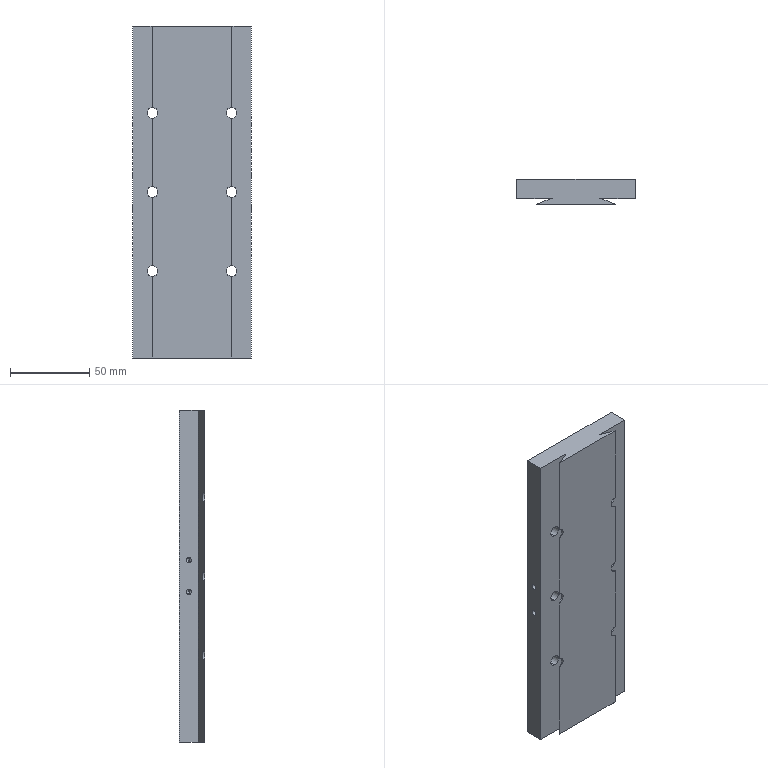Part | SolidWorks | features HoleWzd 2, Extrusion 1, LPattern 1, MirrorPattern 1 | 1 solid | 44 faces | box 75 x 16 x 210 mm | volume 219565 mm3 | cylinder 26 | plane 10 | cone 8 | commonest cylinder face diameters 6.8 x18 3.3 x8
STEP:
#1=CARTESIAN_POINT('',(25.,-6.,46.6));
#2=VERTEX_POINT('',#1);
#3=CARTESIAN_POINT('',(25.,-6.,53.4));
#4=VERTEX_POINT('',#3);
#5=CARTESIAN_POINT('',(25.,-6.,50.));
#6=DIRECTION('',(0.,1.,0.));
#7=DIRECTION('',(0.,0.,1.));
#8=AXIS2_PLACEMENT_3D('',#5,#6,#7);
#9=CIRCLE('',#8,3.4);
#10=EDGE_CURVE('',#2,#4,#9,.T.);
#11=ORIENTED_EDGE('',*,*,#10,.F.);
#12=CARTESIAN_POINT('',(25.,6.,46.6));
#13=VERTEX_POINT('',#12);
#14=CARTESIAN_POINT('',(25.,6.,46.6));
#15=DIRECTION('',(0.,1.,0.));
#16=VECTOR('',#15,1000.);
#17=LINE('',#14,#16);
#18=EDGE_CURVE('',#2,#13,#17,.T.);
#19=ORIENTED_EDGE('',*,*,#18,.T.);
#20=CARTESIAN_POINT('',(25.,6.,53.4));
#21=VERTEX_POINT('',#20);
#22=CARTESIAN_POINT('',(25.,6.,50.));
#23=DIRECTION('',(0.,1.,0.));
#24=DIRECTION('',(0.,0.,1.));
#25=AXIS2_PLACEMENT_3D('',#22,#23,#24);
#26=CIRCLE('',#25,3.4);
#27=EDGE_CURVE('',#13,#21,#26,.T.);
#28=ORIENTED_EDGE('',*,*,#27,.T.);
#29=CARTESIAN_POINT('',(25.,6.,53.4));
#30=DIRECTION('',(0.,1.,0.));
#31=VECTOR('',#30,1000.);
#32=LINE('',#29,#31);
#33=EDGE_CURVE('',#4,#21,#32,.T.);
#34=ORIENTED_EDGE('',*,*,#33,.F.);
#35=EDGE_LOOP('',(#11,#19,#28,#34));
#36=FACE_OUTER_BOUND('',#35,.T.);
#37=CARTESIAN_POINT('',(25.,6.,50.));
#38=DIRECTION('',(0.,1.,0.));
#39=DIRECTION('',(0.,0.,1.));
#40=AXIS2_PLACEMENT_3D('',#37,#38,#39);
#41=CYLINDRICAL_SURFACE('',#40,3.4);
#42=ADVANCED_FACE('',(#36),#41,.F.);
#43=CARTESIAN_POINT('',(-25.,-6.,46.6));
#44=VERTEX_POINT('',#43);
#45=CARTESIAN_POINT('',(-25.,-6.,53.4));
#46=VERTEX_POINT('',#45);
#47=CARTESIAN_POINT('',(-25.,-6.,50.));
#48=DIRECTION('',(0.,1.,0.));
#49=DIRECTION('',(0.,0.,1.));
#50=AXIS2_PLACEMENT_3D('',#47,#48,#49);
#51=CIRCLE('',#50,3.4);
#52=EDGE_CURVE('',#44,#46,#51,.T.);
#53=ORIENTED_EDGE('',*,*,#52,.F.);
#54=CARTESIAN_POINT('',(-25.,6.,46.6));
#55=VERTEX_POINT('',#54);
#56=CARTESIAN_POINT('',(-25.,6.,46.6));
#57=DIRECTION('',(0.,1.,0.));
#58=VECTOR('',#57,1000.);
#59=LINE('',#56,#58);
#60=EDGE_CURVE('',#44,#55,#59,.T.);
#61=ORIENTED_EDGE('',*,*,#60,.T.);
#62=CARTESIAN_POINT('',(-25.,6.,53.4));
#63=VERTEX_POINT('',#62);
#64=CARTESIAN_POINT('',(-25.,6.,50.));
#65=DIRECTION('',(0.,1.,0.));
#66=DIRECTION('',(0.,0.,1.));
#67=AXIS2_PLACEMENT_3D('',#64,#65,#66);
#68=CIRCLE('',#67,3.4);
#69=EDGE_CURVE('',#55,#63,#68,.T.);
#70=ORIENTED_EDGE('',*,*,#69,.T.);
#71=CARTESIAN_POINT('',(-25.,6.,53.4));
#72=DIRECTION('',(0.,1.,0.));
#73=VECTOR('',#72,1000.);
#74=LINE('',#71,#73);
#75=EDGE_CURVE('',#46,#63,#74,.T.);
#76=ORIENTED_EDGE('',*,*,#75,.F.);
#77=EDGE_LOOP('',(#53,#61,#70,#76));
#78=FACE_OUTER_BOUND('',#77,.T.);
#79=CARTESIAN_POINT('',(-25.,6.,50.));
#80=DIRECTION('',(0.,1.,0.));
#81=DIRECTION('',(0.,0.,1.));
#82=AXIS2_PLACEMENT_3D('',#79,#80,#81);
#83=CYLINDRICAL_SURFACE('',#82,3.4);
#84=ADVANCED_FACE('',(#78),#83,.F.);
#85=CARTESIAN_POINT('',(25.,-6.,-3.4));
#86=VERTEX_POINT('',#85);
#87=CARTESIAN_POINT('',(25.,-6.,3.4));
#88=VERTEX_POINT('',#87);
#89=CARTESIAN_POINT('',(25.,-6.,0.));
#90=DIRECTION('',(0.,1.,0.));
#91=DIRECTION('',(0.,0.,1.));
#92=AXIS2_PLACEMENT_3D('',#89,#90,#91);
#93=CIRCLE('',#92,3.4);
#94=EDGE_CURVE('',#86,#88,#93,.T.);
#95=ORIENTED_EDGE('',*,*,#94,.F.);
#96=CARTESIAN_POINT('',(25.,6.,-3.4));
#97=VERTEX_POINT('',#96);
#98=CARTESIAN_POINT('',(25.,6.,-3.4));
#99=DIRECTION('',(0.,1.,0.));
#100=VECTOR('',#99,1000.);
#101=LINE('',#98,#100);
#102=EDGE_CURVE('',#86,#97,#101,.T.);
#103=ORIENTED_EDGE('',*,*,#102,.T.);
#104=CARTESIAN_POINT('',(25.,6.,3.4));
#105=VERTEX_POINT('',#104);
#106=CARTESIAN_POINT('',(25.,6.,0.));
#107=DIRECTION('',(0.,1.,0.));
#108=DIRECTION('',(0.,0.,1.));
#109=AXIS2_PLACEMENT_3D('',#106,#107,#108);
#110=CIRCLE('',#109,3.4);
#111=EDGE_CURVE('',#97,#105,#110,.T.);
#112=ORIENTED_EDGE('',*,*,#111,.T.);
#113=CARTESIAN_POINT('',(25.,6.,3.4));
#114=DIRECTION('',(0.,1.,0.));
#115=VECTOR('',#114,1000.);
#116=LINE('',#113,#115);
#117=EDGE_CURVE('',#88,#105,#116,.T.);
#118=ORIENTED_EDGE('',*,*,#117,.F.);
#119=EDGE_LOOP('',(#95,#103,#112,#118));
#120=FACE_OUTER_BOUND('',#119,.T.);
#121=CARTESIAN_POINT('',(25.,6.,0.));
#122=DIRECTION('',(0.,1.,0.));
#123=DIRECTION('',(0.,0.,1.));
#124=AXIS2_PLACEMENT_3D('',#121,#122,#123);
#125=CYLINDRICAL_SURFACE('',#124,3.4);
#126=ADVANCED_FACE('',(#120),#125,.F.);
#127=CARTESIAN_POINT('',(-25.,-6.,-3.4));
#128=VERTEX_POINT('',#127);
#129=CARTESIAN_POINT('',(-25.,-6.,3.4));
#130=VERTEX_POINT('',#129);
#131=CARTESIAN_POINT('',(-25.,-6.,0.));
#132=DIRECTION('',(0.,1.,0.));
#133=DIRECTION('',(0.,0.,1.));
#134=AXIS2_PLACEMENT_3D('',#131,#132,#133);
#135=CIRCLE('',#134,3.4);
#136=EDGE_CURVE('',#128,#130,#135,.T.);
#137=ORIENTED_EDGE('',*,*,#136,.F.);
#138=CARTESIAN_POINT('',(-25.,6.,-3.4));
#139=VERTEX_POINT('',#138);
#140=CARTESIAN_POINT('',(-25.,6.,-3.4));
#141=DIRECTION('',(0.,1.,0.));
#142=VECTOR('',#141,1000.);
#143=LINE('',#140,#142);
#144=EDGE_CURVE('',#128,#139,#143,.T.);
#145=ORIENTED_EDGE('',*,*,#144,.T.);
#146=CARTESIAN_POINT('',(-25.,6.,3.4));
#147=VERTEX_POINT('',#146);
#148=CARTESIAN_POINT('',(-25.,6.,0.));
#149=DIRECTION('',(0.,1.,0.));
#150=DIRECTION('',(0.,0.,1.));
#151=AXIS2_PLACEMENT_3D('',#148,#149,#150);
#152=CIRCLE('',#151,3.4);
#153=EDGE_CURVE('',#139,#147,#152,.T.);
#154=ORIENTED_EDGE('',*,*,#153,.T.);
#155=CARTESIAN_POINT('',(-25.,6.,3.4));
#156=DIRECTION('',(0.,1.,0.));
#157=VECTOR('',#156,1000.);
#158=LINE('',#155,#157);
#159=EDGE_CURVE('',#130,#147,#158,.T.);
#160=ORIENTED_EDGE('',*,*,#159,.F.);
#161=EDGE_LOOP('',(#137,#145,#154,#160));
#162=FACE_OUTER_BOUND('',#161,.T.);
#163=CARTESIAN_POINT('',(-25.,6.,0.));
#164=DIRECTION('',(0.,1.,0.));
#165=DIRECTION('',(0.,0.,1.));
#166=AXIS2_PLACEMENT_3D('',#163,#164,#165);
#167=CYLINDRICAL_SURFACE('',#166,3.4);
#168=ADVANCED_FACE('',(#162),#167,.F.);
#169=CARTESIAN_POINT('',(25.,-6.,-53.4));
#170=VERTEX_POINT('',#169);
#171=CARTESIAN_POINT('',(25.,-6.,-46.6));
#172=VERTEX_POINT('',#171);
#173=CARTESIAN_POINT('',(25.,-6.,-50.));
#174=DIRECTION('',(0.,1.,0.));
#175=DIRECTION('',(0.,0.,1.));
#176=AXIS2_PLACEMENT_3D('',#173,#174,#175);
#177=CIRCLE('',#176,3.4);
#178=EDGE_CURVE('',#170,#172,#177,.T.);
#179=ORIENTED_EDGE('',*,*,#178,.F.);
#180=CARTESIAN_POINT('',(25.,6.,-53.4));
#181=VERTEX_POINT('',#180);
#182=CARTESIAN_POINT('',(25.,6.,-53.4));
#183=DIRECTION('',(0.,1.,0.));
#184=VECTOR('',#183,1000.);
#185=LINE('',#182,#184);
#186=EDGE_CURVE('',#170,#181,#185,.T.);
#187=ORIENTED_EDGE('',*,*,#186,.T.);
#188=CARTESIAN_POINT('',(25.,6.,-46.6));
#189=VERTEX_POINT('',#188);
#190=CARTESIAN_POINT('',(25.,6.,-50.));
#191=DIRECTION('',(0.,1.,0.));
#192=DIRECTION('',(0.,0.,1.));
#193=AXIS2_PLACEMENT_3D('',#190,#191,#192);
#194=CIRCLE('',#193,3.4);
#195=EDGE_CURVE('',#181,#189,#194,.T.);
#196=ORIENTED_EDGE('',*,*,#195,.T.);
#197=CARTESIAN_POINT('',(25.,6.,-46.6));
#198=DIRECTION('',(0.,1.,0.));
#199=VECTOR('',#198,1000.);
#200=LINE('',#197,#199);
#201=EDGE_CURVE('',#172,#189,#200,.T.);
#202=ORIENTED_EDGE('',*,*,#201,.F.);
#203=EDGE_LOOP('',(#179,#187,#196,#202));
#204=FACE_OUTER_BOUND('',#203,.T.);
#205=CARTESIAN_POINT('',(25.,6.,-50.));
#206=DIRECTION('',(0.,1.,0.));
#207=DIRECTION('',(0.,0.,1.));
#208=AXIS2_PLACEMENT_3D('',#205,#206,#207);
#209=CYLINDRICAL_SURFACE('',#208,3.4);
#210=ADVANCED_FACE('',(#204),#209,.F.);
#211=CARTESIAN_POINT('',(-25.,-6.,-53.4));
#212=VERTEX_POINT('',#211);
#213=CARTESIAN_POINT('',(-25.,-6.,-46.6));
#214=VERTEX_POINT('',#213);
#215=CARTESIAN_POINT('',(-25.,-6.,-50.));
#216=DIRECTION('',(0.,1.,0.));
#217=DIRECTION('',(0.,0.,1.));
#218=AXIS2_PLACEMENT_3D('',#215,#216,#217);
#219=CIRCLE('',#218,3.4);
#220=EDGE_CURVE('',#212,#214,#219,.T.);
#221=ORIENTED_EDGE('',*,*,#220,.F.);
#222=CARTESIAN_POINT('',(-25.,6.,-53.4));
#223=VERTEX_POINT('',#222);
#224=CARTESIAN_POINT('',(-25.,6.,-53.4));
#225=DIRECTION('',(0.,1.,0.));
#226=VECTOR('',#225,1000.);
#227=LINE('',#224,#226);
#228=EDGE_CURVE('',#212,#223,#227,.T.);
#229=ORIENTED_EDGE('',*,*,#228,.T.);
#230=CARTESIAN_POINT('',(-25.,6.,-46.6));
#231=VERTEX_POINT('',#230);
#232=CARTESIAN_POINT('',(-25.,6.,-50.));
#233=DIRECTION('',(0.,1.,0.));
#234=DIRECTION('',(0.,0.,1.));
#235=AXIS2_PLACEMENT_3D('',#232,#233,#234);
#236=CIRCLE('',#235,3.4);
#237=EDGE_CURVE('',#223,#231,#236,.T.);
#238=ORIENTED_EDGE('',*,*,#237,.T.);
#239=CARTESIAN_POINT('',(-25.,6.,-46.6));
#240=DIRECTION('',(0.,1.,0.));
#241=VECTOR('',#240,1000.);
#242=LINE('',#239,#241);
#243=EDGE_CURVE('',#214,#231,#242,.T.);
#244=ORIENTED_EDGE('',*,*,#243,.F.);
#245=EDGE_LOOP('',(#221,#229,#238,#244));
#246=FACE_OUTER_BOUND('',#245,.T.);
#247=CARTESIAN_POINT('',(-25.,6.,-50.));
#248=DIRECTION('',(0.,1.,0.));
#249=DIRECTION('',(0.,0.,1.));
#250=AXIS2_PLACEMENT_3D('',#247,#248,#249);
#251=CYLINDRICAL_SURFACE('',#250,3.4);
#252=ADVANCED_FACE('',(#246),#251,.F.);
#253=CARTESIAN_POINT('',(27.4,0.,-8.35));
#254=VERTEX_POINT('',#253);
#255=CARTESIAN_POINT('',(27.4,0.,-11.65));
#256=VERTEX_POINT('',#255);
#257=CARTESIAN_POINT('',(27.4,0.,-10.));
#258=DIRECTION('',(1.,0.,0.));
#259=DIRECTION('',(0.,0.,-1.));
#260=AXIS2_PLACEMENT_3D('',#257,#258,#259);
#261=CIRCLE('',#260,1.65);
#262=EDGE_CURVE('',#254,#256,#261,.T.);
#263=ORIENTED_EDGE('',*,*,#262,.F.);
#264=CARTESIAN_POINT('',(37.5,0.,-8.35));
#265=VERTEX_POINT('',#264);
#266=CARTESIAN_POINT('',(37.5,0.,-8.35));
#267=DIRECTION('',(1.,0.,0.));
#268=VECTOR('',#267,1000.);
#269=LINE('',#266,#268);
#270=EDGE_CURVE('',#254,#265,#269,.T.);
#271=ORIENTED_EDGE('',*,*,#270,.T.);
#272=CARTESIAN_POINT('',(37.5,0.,-11.65));
#273=VERTEX_POINT('',#272);
#274=CARTESIAN_POINT('',(37.5,0.,-10.));
#275=DIRECTION('',(1.,0.,0.));
#276=DIRECTION('',(0.,0.,-1.));
#277=AXIS2_PLACEMENT_3D('',#274,#275,#276);
#278=CIRCLE('',#277,1.65);
#279=EDGE_CURVE('',#265,#273,#278,.T.);
#280=ORIENTED_EDGE('',*,*,#279,.T.);
#281=CARTESIAN_POINT('',(37.5,0.,-11.65));
#282=DIRECTION('',(1.,0.,0.));
#283=VECTOR('',#282,1000.);
#284=LINE('',#281,#283);
#285=EDGE_CURVE('',#256,#273,#284,.T.);
#286=ORIENTED_EDGE('',*,*,#285,.F.);
#287=EDGE_LOOP('',(#263,#271,#280,#286));
#288=FACE_OUTER_BOUND('',#287,.T.);
#289=CARTESIAN_POINT('',(37.5,0.,-10.));
#290=DIRECTION('',(1.,0.,0.));
#291=DIRECTION('',(0.,0.,-1.));
#292=AXIS2_PLACEMENT_3D('',#289,#290,#291);
#293=CYLINDRICAL_SURFACE('',#292,1.65);
#294=ADVANCED_FACE('',(#288),#293,.F.);
#295=CARTESIAN_POINT('',(26.409,0.,-10.));
#296=VERTEX_POINT('',#295);
#297=CARTESIAN_POINT('',(27.4,0.,-11.65));
#298=DIRECTION('',(0.515,0.,-0.8572));
#299=VECTOR('',#298,1000.);
#300=LINE('',#297,#299);
#301=EDGE_CURVE('',#296,#256,#300,.T.);
#302=ORIENTED_EDGE('',*,*,#301,.F.);
#303=CARTESIAN_POINT('',(27.4,0.,-8.35));
#304=DIRECTION('',(0.515,0.,0.8572));
#305=VECTOR('',#304,1000.);
#306=LINE('',#303,#305);
#307=EDGE_CURVE('',#296,#254,#306,.T.);
#308=ORIENTED_EDGE('',*,*,#307,.T.);
#309=ORIENTED_EDGE('',*,*,#262,.T.);
#310=EDGE_LOOP('',(#302,#308,#309));
#311=FACE_OUTER_BOUND('',#310,.T.);
#312=CARTESIAN_POINT('',(27.4,0.,-10.));
#313=DIRECTION('',(1.,0.,0.));
#314=DIRECTION('',(0.,0.,-1.));
#315=AXIS2_PLACEMENT_3D('',#312,#313,#314);
#316=CONICAL_SURFACE('',#315,1.65,1.03);
#317=ADVANCED_FACE('',(#311),#316,.F.);
#318=CARTESIAN_POINT('',(27.4,0.,11.65));
#319=VERTEX_POINT('',#318);
#320=CARTESIAN_POINT('',(27.4,0.,8.35));
#321=VERTEX_POINT('',#320);
#322=CARTESIAN_POINT('',(27.4,0.,10.));
#323=DIRECTION('',(1.,0.,0.));
#324=DIRECTION('',(0.,0.,-1.));
#325=AXIS2_PLACEMENT_3D('',#322,#323,#324);
#326=CIRCLE('',#325,1.65);
#327=EDGE_CURVE('',#319,#321,#326,.T.);
#328=ORIENTED_EDGE('',*,*,#327,.F.);
#329=CARTESIAN_POINT('',(37.5,0.,11.65));
#330=VERTEX_POINT('',#329);
#331=CARTESIAN_POINT('',(37.5,0.,11.65));
#332=DIRECTION('',(1.,0.,0.));
#333=VECTOR('',#332,1000.);
#334=LINE('',#331,#333);
#335=EDGE_CURVE('',#319,#330,#334,.T.);
#336=ORIENTED_EDGE('',*,*,#335,.T.);
#337=CARTESIAN_POINT('',(37.5,0.,8.35));
#338=VERTEX_POINT('',#337);
#339=CARTESIAN_POINT('',(37.5,0.,10.));
#340=DIRECTION('',(1.,0.,0.));
#341=DIRECTION('',(0.,0.,-1.));
#342=AXIS2_PLACEMENT_3D('',#339,#340,#341);
#343=CIRCLE('',#342,1.65);
#344=EDGE_CURVE('',#330,#338,#343,.T.);
#345=ORIENTED_EDGE('',*,*,#344,.T.);
#346=CARTESIAN_POINT('',(37.5,0.,8.35));
#347=DIRECTION('',(1.,0.,0.));
#348=VECTOR('',#347,1000.);
#349=LINE('',#346,#348);
#350=EDGE_CURVE('',#321,#338,#349,.T.);
#351=ORIENTED_EDGE('',*,*,#350,.F.);
#352=EDGE_LOOP('',(#328,#336,#345,#351));
#353=FACE_OUTER_BOUND('',#352,.T.);
#354=CARTESIAN_POINT('',(37.5,0.,10.));
#355=DIRECTION('',(1.,0.,0.));
#356=DIRECTION('',(0.,0.,-1.));
#357=AXIS2_PLACEMENT_3D('',#354,#355,#356);
#358=CYLINDRICAL_SURFACE('',#357,1.65);
#359=ADVANCED_FACE('',(#353),#358,.F.);
#360=CARTESIAN_POINT('',(26.409,0.,10.));
#361=VERTEX_POINT('',#360);
#362=CARTESIAN_POINT('',(27.4,0.,8.35));
#363=DIRECTION('',(0.515,0.,-0.8572));
#364=VECTOR('',#363,1000.);
#365=LINE('',#362,#364);
#366=EDGE_CURVE('',#361,#321,#365,.T.);
#367=ORIENTED_EDGE('',*,*,#366,.F.);
#368=CARTESIAN_POINT('',(27.4,0.,11.65));
#369=DIRECTION('',(0.515,0.,0.8572));
#370=VECTOR('',#369,1000.);
#371=LINE('',#368,#370);
#372=EDGE_CURVE('',#361,#319,#371,.T.);
#373=ORIENTED_EDGE('',*,*,#372,.T.);
#374=ORIENTED_EDGE('',*,*,#327,.T.);
#375=EDGE_LOOP('',(#367,#373,#374));
#376=FACE_OUTER_BOUND('',#375,.T.);
#377=CARTESIAN_POINT('',(27.4,0.,10.));
#378=DIRECTION('',(1.,0.,0.));
#379=DIRECTION('',(0.,0.,-1.));
#380=AXIS2_PLACEMENT_3D('',#377,#378,#379);
#381=CONICAL_SURFACE('',#380,1.65,1.03);
#382=ADVANCED_FACE('',(#376),#381,.F.);
#383=CARTESIAN_POINT('',(-27.4,0.,-11.65));
#384=VERTEX_POINT('',#383);
#385=CARTESIAN_POINT('',(-27.4,0.,-8.35));
#386=VERTEX_POINT('',#385);
#387=CARTESIAN_POINT('',(-27.4,0.,-10.));
#388=DIRECTION('',(-1.,0.,0.));
#389=DIRECTION('',(0.,0.,1.));
#390=AXIS2_PLACEMENT_3D('',#387,#388,#389);
#391=CIRCLE('',#390,1.65);
#392=EDGE_CURVE('',#384,#386,#391,.T.);
#393=ORIENTED_EDGE('',*,*,#392,.F.);
#394=CARTESIAN_POINT('',(-37.5,0.,-11.65));
#395=VERTEX_POINT('',#394);
#396=CARTESIAN_POINT('',(-37.5,0.,-11.65));
#397=DIRECTION('',(-1.,0.,0.));
#398=VECTOR('',#397,1000.);
#399=LINE('',#396,#398);
#400=EDGE_CURVE('',#384,#395,#399,.T.);
#401=ORIENTED_EDGE('',*,*,#400,.T.);
#402=CARTESIAN_POINT('',(-37.5,0.,-8.35));
#403=VERTEX_POINT('',#402);
#404=CARTESIAN_POINT('',(-37.5,0.,-10.));
#405=DIRECTION('',(-1.,0.,0.));
#406=DIRECTION('',(0.,0.,1.));
#407=AXIS2_PLACEMENT_3D('',#404,#405,#406);
#408=CIRCLE('',#407,1.65);
#409=EDGE_CURVE('',#395,#403,#408,.T.);
#410=ORIENTED_EDGE('',*,*,#409,.T.);
#411=CARTESIAN_POINT('',(-37.5,0.,-8.35));
#412=DIRECTION('',(-1.,0.,0.));
#413=VECTOR('',#412,1000.);
#414=LINE('',#411,#413);
#415=EDGE_CURVE('',#386,#403,#414,.T.);
#416=ORIENTED_EDGE('',*,*,#415,.F.);
#417=EDGE_LOOP('',(#393,#401,#410,#416));
#418=FACE_OUTER_BOUND('',#417,.T.);
#419=CARTESIAN_POINT('',(-37.5,0.,-10.));
#420=DIRECTION('',(-1.,0.,0.));
#421=DIRECTION('',(0.,0.,1.));
#422=AXIS2_PLACEMENT_3D('',#419,#420,#421);
#423=CYLINDRICAL_SURFACE('',#422,1.65);
#424=ADVANCED_FACE('',(#418),#423,.F.);
#425=CARTESIAN_POINT('',(-26.409,0.,-10.));
#426=VERTEX_POINT('',#425);
#427=CARTESIAN_POINT('',(-27.4,0.,-8.35));
#428=DIRECTION('',(-0.515,0.,0.8572));
#429=VECTOR('',#428,1000.);
#430=LINE('',#427,#429);
#431=EDGE_CURVE('',#426,#386,#430,.T.);
#432=ORIENTED_EDGE('',*,*,#431,.F.);
#433=CARTESIAN_POINT('',(-27.4,0.,-11.65));
#434=DIRECTION('',(-0.515,0.,-0.8572));
#435=VECTOR('',#434,1000.);
#436=LINE('',#433,#435);
#437=EDGE_CURVE('',#426,#384,#436,.T.);
#438=ORIENTED_EDGE('',*,*,#437,.T.);
#439=ORIENTED_EDGE('',*,*,#392,.T.);
#440=EDGE_LOOP('',(#432,#438,#439));
#441=FACE_OUTER_BOUND('',#440,.T.);
#442=CARTESIAN_POINT('',(-27.4,0.,-10.));
#443=DIRECTION('',(-1.,0.,0.));
#444=DIRECTION('',(0.,0.,1.));
#445=AXIS2_PLACEMENT_3D('',#442,#443,#444);
#446=CONICAL_SURFACE('',#445,1.65,1.03);
#447=ADVANCED_FACE('',(#441),#446,.F.);
#448=CARTESIAN_POINT('',(-27.4,0.,8.35));
#449=VERTEX_POINT('',#448);
#450=CARTESIAN_POINT('',(-27.4,0.,11.65));
#451=VERTEX_POINT('',#450);
#452=CARTESIAN_POINT('',(-27.4,0.,10.));
#453=DIRECTION('',(-1.,0.,0.));
#454=DIRECTION('',(0.,0.,1.));
#455=AXIS2_PLACEMENT_3D('',#452,#453,#454);
#456=CIRCLE('',#455,1.65);
#457=EDGE_CURVE('',#449,#451,#456,.T.);
#458=ORIENTED_EDGE('',*,*,#457,.F.);
#459=CARTESIAN_POINT('',(-37.5,0.,8.35));
#460=VERTEX_POINT('',#459);
#461=CARTESIAN_POINT('',(-37.5,0.,8.35));
#462=DIRECTION('',(-1.,0.,0.));
#463=VECTOR('',#462,1000.);
#464=LINE('',#461,#463);
#465=EDGE_CURVE('',#449,#460,#464,.T.);
#466=ORIENTED_EDGE('',*,*,#465,.T.);
#467=CARTESIAN_POINT('',(-37.5,0.,11.65));
#468=VERTEX_POINT('',#467);
#469=CARTESIAN_POINT('',(-37.5,0.,10.));
#470=DIRECTION('',(-1.,0.,0.));
#471=DIRECTION('',(0.,0.,1.));
#472=AXIS2_PLACEMENT_3D('',#469,#470,#471);
#473=CIRCLE('',#472,1.65);
#474=EDGE_CURVE('',#460,#468,#473,.T.);
#475=ORIENTED_EDGE('',*,*,#474,.T.);
#476=CARTESIAN_POINT('',(-37.5,0.,11.65));
#477=DIRECTION('',(-1.,0.,0.));
#478=VECTOR('',#477,1000.);
#479=LINE('',#476,#478);
#480=EDGE_CURVE('',#451,#468,#479,.T.);
#481=ORIENTED_EDGE('',*,*,#480,.F.);
#482=EDGE_LOOP('',(#458,#466,#475,#481));
#483=FACE_OUTER_BOUND('',#482,.T.);
#484=CARTESIAN_POINT('',(-37.5,0.,10.));
#485=DIRECTION('',(-1.,0.,0.));
#486=DIRECTION('',(0.,0.,1.));
#487=AXIS2_PLACEMENT_3D('',#484,#485,#486);
#488=CYLINDRICAL_SURFACE('',#487,1.65);
#489=ADVANCED_FACE('',(#483),#488,.F.);
#490=CARTESIAN_POINT('',(-26.409,0.,10.));
#491=VERTEX_POINT('',#490);
#492=CARTESIAN_POINT('',(-27.4,0.,11.65));
#493=DIRECTION('',(-0.515,0.,0.8572));
#494=VECTOR('',#493,1000.);
#495=LINE('',#492,#494);
#496=EDGE_CURVE('',#491,#451,#495,.T.);
#497=ORIENTED_EDGE('',*,*,#496,.F.);
#498=CARTESIAN_POINT('',(-27.4,0.,8.35));
#499=DIRECTION('',(-0.515,0.,-0.8572));
#500=VECTOR('',#499,1000.);
#501=LINE('',#498,#500);
#502=EDGE_CURVE('',#491,#449,#501,.T.);
#503=ORIENTED_EDGE('',*,*,#502,.T.);
#504=ORIENTED_EDGE('',*,*,#457,.T.);
#505=EDGE_LOOP('',(#497,#503,#504));
#506=FACE_OUTER_BOUND('',#505,.T.);
#507=CARTESIAN_POINT('',(-27.4,0.,10.));
#508=DIRECTION('',(-1.,0.,0.));
#509=DIRECTION('',(0.,0.,1.));
#510=AXIS2_PLACEMENT_3D('',#507,#508,#509);
#511=CONICAL_SURFACE('',#510,1.65,1.03);
#512=ADVANCED_FACE('',(#506),#511,.F.);
#513=CARTESIAN_POINT('',(25.,-6.,50.));
#514=DIRECTION('',(0.,1.,0.));
#515=DIRECTION('',(0.,0.,1.));
#516=AXIS2_PLACEMENT_3D('',#513,#514,#515);
#517=CIRCLE('',#516,3.4);
#518=EDGE_CURVE('',#4,#2,#517,.T.);
#519=ORIENTED_EDGE('',*,*,#518,.T.);
#520=ORIENTED_EDGE('',*,*,#10,.T.);
#521=EDGE_LOOP('',(#519,#520));
#522=FACE_BOUND('',#521,.T.);
#523=CARTESIAN_POINT('',(25.,-6.,0.));
#524=DIRECTION('',(0.,1.,0.));
#525=DIRECTION('',(0.,0.,1.));
#526=AXIS2_PLACEMENT_3D('',#523,#524,#525);
#527=CIRCLE('',#526,3.4);
#528=EDGE_CURVE('',#88,#86,#527,.T.);
#529=ORIENTED_EDGE('',*,*,#528,.T.);
#530=ORIENTED_EDGE('',*,*,#94,.T.);
#531=EDGE_LOOP('',(#529,#530));
#532=FACE_BOUND('',#531,.T.);
#533=CARTESIAN_POINT('',(25.,-6.,-50.));
#534=DIRECTION('',(0.,1.,0.));
#535=DIRECTION('',(0.,0.,1.));
#536=AXIS2_PLACEMENT_3D('',#533,#534,#535);
#537=CIRCLE('',#536,3.4);
#538=EDGE_CURVE('',#172,#170,#537,.T.);
#539=ORIENTED_EDGE('',*,*,#538,.T.);
#540=ORIENTED_EDGE('',*,*,#178,.T.);
#541=EDGE_LOOP('',(#539,#540));
#542=FACE_BOUND('',#541,.T.);
#543=CARTESIAN_POINT('',(15.,-6.,-105.));
#544=VERTEX_POINT('',#543);
#545=CARTESIAN_POINT('',(37.5,-6.,-105.));
#546=VERTEX_POINT('',#545);
#547=CARTESIAN_POINT('',(15.,-6.,-105.));
#548=DIRECTION('',(1.,0.,0.));
#549=VECTOR('',#548,1000.);
#550=LINE('',#547,#549);
#551=EDGE_CURVE('',#544,#546,#550,.T.);
#552=ORIENTED_EDGE('',*,*,#551,.T.);
#553=CARTESIAN_POINT('',(37.5,-6.,105.));
#554=VERTEX_POINT('',#553);
#555=CARTESIAN_POINT('',(37.5,-6.,105.));
#556=DIRECTION('',(0.,0.,-1.));
#557=VECTOR('',#556,1000.);
#558=LINE('',#555,#557);
#559=EDGE_CURVE('',#554,#546,#558,.T.);
#560=ORIENTED_EDGE('',*,*,#559,.F.);
#561=CARTESIAN_POINT('',(15.,-6.,105.));
#562=VERTEX_POINT('',#561);
#563=CARTESIAN_POINT('',(15.,-6.,105.));
#564=DIRECTION('',(1.,0.,0.));
#565=VECTOR('',#564,1000.);
#566=LINE('',#563,#565);
#567=EDGE_CURVE('',#562,#554,#566,.T.);
#568=ORIENTED_EDGE('',*,*,#567,.F.);
#569=CARTESIAN_POINT('',(15.,-6.,105.));
#570=DIRECTION('',(0.,0.,-1.));
#571=VECTOR('',#570,1000.);
#572=LINE('',#569,#571);
#573=EDGE_CURVE('',#562,#544,#572,.T.);
#574=ORIENTED_EDGE('',*,*,#573,.T.);
#575=EDGE_LOOP('',(#552,#560,#568,#574));
#576=FACE_OUTER_BOUND('',#575,.T.);
#577=CARTESIAN_POINT('',(15.,-6.,105.));
#578=DIRECTION('',(0.,1.,0.));
#579=DIRECTION('',(0.,0.,1.));
#580=AXIS2_PLACEMENT_3D('',#577,#578,#579);
#581=PLANE('',#580);
#582=ADVANCED_FACE('',(#522,#532,#542,#576),#581,.F.);
#583=CARTESIAN_POINT('',(37.5,0.,-10.));
#584=DIRECTION('',(1.,0.,0.));
#585=DIRECTION('',(0.,0.,-1.));
#586=AXIS2_PLACEMENT_3D('',#583,#584,#585);
#587=CIRCLE('',#586,1.65);
#588=EDGE_CURVE('',#273,#265,#587,.T.);
#589=ORIENTED_EDGE('',*,*,#588,.F.);
#590=ORIENTED_EDGE('',*,*,#279,.F.);
#591=EDGE_LOOP('',(#589,#590));
#592=FACE_BOUND('',#591,.T.);
#593=CARTESIAN_POINT('',(37.5,0.,10.));
#594=DIRECTION('',(1.,0.,0.));
#595=DIRECTION('',(0.,0.,-1.));
#596=AXIS2_PLACEMENT_3D('',#593,#594,#595);
#597=CIRCLE('',#596,1.65);
#598=EDGE_CURVE('',#338,#330,#597,.T.);
#599=ORIENTED_EDGE('',*,*,#598,.F.);
#600=ORIENTED_EDGE('',*,*,#344,.F.);
#601=EDGE_LOOP('',(#599,#600));
#602=FACE_BOUND('',#601,.T.);
#603=CARTESIAN_POINT('',(37.5,6.,-105.));
#604=VERTEX_POINT('',#603);
#605=CARTESIAN_POINT('',(37.5,6.,-105.));
#606=DIRECTION('',(0.,1.,0.));
#607=VECTOR('',#606,1000.);
#608=LINE('',#605,#607);
#609=EDGE_CURVE('',#546,#604,#608,.T.);
#610=ORIENTED_EDGE('',*,*,#609,.T.);
#611=CARTESIAN_POINT('',(37.5,6.,105.));
#612=VERTEX_POINT('',#611);
#613=CARTESIAN_POINT('',(37.5,6.,105.));
#614=DIRECTION('',(0.,0.,-1.));
#615=VECTOR('',#614,1000.);
#616=LINE('',#613,#615);
#617=EDGE_CURVE('',#612,#604,#616,.T.);
#618=ORIENTED_EDGE('',*,*,#617,.F.);
#619=CARTESIAN_POINT('',(37.5,6.,105.));
#620=DIRECTION('',(0.,1.,0.));
#621=VECTOR('',#620,1000.);
#622=LINE('',#619,#621);
#623=EDGE_CURVE('',#554,#612,#622,.T.);
#624=ORIENTED_EDGE('',*,*,#623,.F.);
#625=ORIENTED_EDGE('',*,*,#559,.T.);
#626=EDGE_LOOP('',(#610,#618,#624,#625));
#627=FACE_OUTER_BOUND('',#626,.T.);
#628=CARTESIAN_POINT('',(37.5,6.,105.));
#629=DIRECTION('',(-1.,0.,0.));
#630=DIRECTION('',(0.,-1.,0.));
#631=AXIS2_PLACEMENT_3D('',#628,#629,#630);
#632=PLANE('',#631);
#633=ADVANCED_FACE('',(#592,#602,#627),#632,.F.);
#634=CARTESIAN_POINT('',(25.,6.,50.));
#635=DIRECTION('',(0.,1.,0.));
#636=DIRECTION('',(0.,0.,1.));
#637=AXIS2_PLACEMENT_3D('',#634,#635,#636);
#638=CIRCLE('',#637,3.4);
#639=EDGE_CURVE('',#21,#13,#638,.T.);
#640=ORIENTED_EDGE('',*,*,#639,.F.);
#641=ORIENTED_EDGE('',*,*,#27,.F.);
#642=EDGE_LOOP('',(#640,#641));
#643=FACE_BOUND('',#642,.T.);
#644=CARTESIAN_POINT('',(-25.,6.,50.));
#645=DIRECTION('',(0.,1.,0.));
#646=DIRECTION('',(0.,0.,1.));
#647=AXIS2_PLACEMENT_3D('',#644,#645,#646);
#648=CIRCLE('',#647,3.4);
#649=EDGE_CURVE('',#63,#55,#648,.T.);
#650=ORIENTED_EDGE('',*,*,#649,.F.);
#651=ORIENTED_EDGE('',*,*,#69,.F.);
#652=EDGE_LOOP('',(#650,#651));
#653=FACE_BOUND('',#652,.T.);
#654=CARTESIAN_POINT('',(25.,6.,0.));
#655=DIRECTION('',(0.,1.,0.));
#656=DIRECTION('',(0.,0.,1.));
#657=AXIS2_PLACEMENT_3D('',#654,#655,#656);
#658=CIRCLE('',#657,3.4);
#659=EDGE_CURVE('',#105,#97,#658,.T.);
#660=ORIENTED_EDGE('',*,*,#659,.F.);
#661=ORIENTED_EDGE('',*,*,#111,.F.);
#662=EDGE_LOOP('',(#660,#661));
#663=FACE_BOUND('',#662,.T.);
#664=CARTESIAN_POINT('',(-25.,6.,0.));
#665=DIRECTION('',(0.,1.,0.));
#666=DIRECTION('',(0.,0.,1.));
#667=AXIS2_PLACEMENT_3D('',#664,#665,#666);
#668=CIRCLE('',#667,3.4);
#669=EDGE_CURVE('',#147,#139,#668,.T.);
#670=ORIENTED_EDGE('',*,*,#669,.F.);
#671=ORIENTED_EDGE('',*,*,#153,.F.);
#672=EDGE_LOOP('',(#670,#671));
#673=FACE_BOUND('',#672,.T.);
#674=CARTESIAN_POINT('',(25.,6.,-50.));
#675=DIRECTION('',(0.,1.,0.));
#676=DIRECTION('',(0.,0.,1.));
#677=AXIS2_PLACEMENT_3D('',#674,#675,#676);
#678=CIRCLE('',#677,3.4);
#679=EDGE_CURVE('',#189,#181,#678,.T.);
#680=ORIENTED_EDGE('',*,*,#679,.F.);
#681=ORIENTED_EDGE('',*,*,#195,.F.);
#682=EDGE_LOOP('',(#680,#681));
#683=FACE_BOUND('',#682,.T.);
#684=CARTESIAN_POINT('',(-25.,6.,-50.));
#685=DIRECTION('',(0.,1.,0.));
#686=DIRECTION('',(0.,0.,1.));
#687=AXIS2_PLACEMENT_3D('',#684,#685,#686);
#688=CIRCLE('',#687,3.4);
#689=EDGE_CURVE('',#231,#223,#688,.T.);
#690=ORIENTED_EDGE('',*,*,#689,.F.);
#691=ORIENTED_EDGE('',*,*,#237,.F.);
#692=EDGE_LOOP('',(#690,#691));
#693=FACE_BOUND('',#692,.T.);
#694=CARTESIAN_POINT('',(-37.5,6.,-105.));
#695=VERTEX_POINT('',#694);
#696=CARTESIAN_POINT('',(-37.5,6.,-105.));
#697=DIRECTION('',(-1.,0.,0.));
#698=VECTOR('',#697,1000.);
#699=LINE('',#696,#698);
#700=EDGE_CURVE('',#604,#695,#699,.T.);
#701=ORIENTED_EDGE('',*,*,#700,.T.);
#702=CARTESIAN_POINT('',(-37.5,6.,105.));
#703=VERTEX_POINT('',#702);
#704=CARTESIAN_POINT('',(-37.5,6.,105.));
#705=DIRECTION('',(0.,0.,-1.));
#706=VECTOR('',#705,1000.);
#707=LINE('',#704,#706);
#708=EDGE_CURVE('',#703,#695,#707,.T.);
#709=ORIENTED_EDGE('',*,*,#708,.F.);
#710=CARTESIAN_POINT('',(-37.5,6.,105.));
#711=DIRECTION('',(-1.,0.,0.));
#712=VECTOR('',#711,1000.);
#713=LINE('',#710,#712);
#714=EDGE_CURVE('',#612,#703,#713,.T.);
#715=ORIENTED_EDGE('',*,*,#714,.F.);
#716=ORIENTED_EDGE('',*,*,#617,.T.);
#717=EDGE_LOOP('',(#701,#709,#715,#716));
#718=FACE_OUTER_BOUND('',#717,.T.);
#719=CARTESIAN_POINT('',(-37.5,6.,105.));
#720=DIRECTION('',(0.,-1.,0.));
#721=DIRECTION('',(0.,0.,-1.));
#722=AXIS2_PLACEMENT_3D('',#719,#720,#721);
#723=PLANE('',#722);
#724=ADVANCED_FACE('',(#643,#653,#663,#673,#683,#693,#718),#723,.F.);
#725=CARTESIAN_POINT('',(-37.5,0.,-10.));
#726=DIRECTION('',(-1.,0.,0.));
#727=DIRECTION('',(0.,0.,1.));
#728=AXIS2_PLACEMENT_3D('',#725,#726,#727);
#729=CIRCLE('',#728,1.65);
#730=EDGE_CURVE('',#403,#395,#729,.T.);
#731=ORIENTED_EDGE('',*,*,#730,.F.);
#732=ORIENTED_EDGE('',*,*,#409,.F.);
#733=EDGE_LOOP('',(#731,#732));
#734=FACE_BOUND('',#733,.T.);
#735=CARTESIAN_POINT('',(-37.5,0.,10.));
#736=DIRECTION('',(-1.,0.,0.));
#737=DIRECTION('',(0.,0.,1.));
#738=AXIS2_PLACEMENT_3D('',#735,#736,#737);
#739=CIRCLE('',#738,1.65);
#740=EDGE_CURVE('',#468,#460,#739,.T.);
#741=ORIENTED_EDGE('',*,*,#740,.F.);
#742=ORIENTED_EDGE('',*,*,#474,.F.);
#743=EDGE_LOOP('',(#741,#742));
#744=FACE_BOUND('',#743,.T.);
#745=CARTESIAN_POINT('',(-37.5,-6.,-105.));
#746=VERTEX_POINT('',#745);
#747=CARTESIAN_POINT('',(-37.5,6.,-105.));
#748=DIRECTION('',(0.,-1.,0.));
#749=VECTOR('',#748,1000.);
#750=LINE('',#747,#749);
#751=EDGE_CURVE('',#695,#746,#750,.T.);
#752=ORIENTED_EDGE('',*,*,#751,.T.);
#753=CARTESIAN_POINT('',(-37.5,-6.,105.));
#754=VERTEX_POINT('',#753);
#755=CARTESIAN_POINT('',(-37.5,-6.,105.));
#756=DIRECTION('',(0.,0.,-1.));
#757=VECTOR('',#756,1000.);
#758=LINE('',#755,#757);
#759=EDGE_CURVE('',#754,#746,#758,.T.);
#760=ORIENTED_EDGE('',*,*,#759,.F.);
#761=CARTESIAN_POINT('',(-37.5,6.,105.));
#762=DIRECTION('',(0.,-1.,0.));
#763=VECTOR('',#762,1000.);
#764=LINE('',#761,#763);
#765=EDGE_CURVE('',#703,#754,#764,.T.);
#766=ORIENTED_EDGE('',*,*,#765,.F.);
#767=ORIENTED_EDGE('',*,*,#708,.T.);
#768=EDGE_LOOP('',(#752,#760,#766,#767));
#769=FACE_OUTER_BOUND('',#768,.T.);
#770=CARTESIAN_POINT('',(-37.5,6.,105.));
#771=DIRECTION('',(1.,0.,0.));
#772=DIRECTION('',(0.,0.,-1.));
#773=AXIS2_PLACEMENT_3D('',#770,#771,#772);
#774=PLANE('',#773);
#775=ADVANCED_FACE('',(#734,#744,#769),#774,.F.);
#776=CARTESIAN_POINT('',(-25.,-6.,50.));
#777=DIRECTION('',(0.,1.,0.));
#778=DIRECTION('',(0.,0.,1.));
#779=AXIS2_PLACEMENT_3D('',#776,#777,#778);
#780=CIRCLE('',#779,3.4);
#781=EDGE_CURVE('',#46,#44,#780,.T.);
#782=ORIENTED_EDGE('',*,*,#781,.T.);
#783=ORIENTED_EDGE('',*,*,#52,.T.);
#784=EDGE_LOOP('',(#782,#783));
#785=FACE_BOUND('',#784,.T.);
#786=CARTESIAN_POINT('',(-25.,-6.,0.));
#787=DIRECTION('',(0.,1.,0.));
#788=DIRECTION('',(0.,0.,1.));
#789=AXIS2_PLACEMENT_3D('',#786,#787,#788);
#790=CIRCLE('',#789,3.4);
#791=EDGE_CURVE('',#130,#128,#790,.T.);
#792=ORIENTED_EDGE('',*,*,#791,.T.);
#793=ORIENTED_EDGE('',*,*,#136,.T.);
#794=EDGE_LOOP('',(#792,#793));
#795=FACE_BOUND('',#794,.T.);
#796=CARTESIAN_POINT('',(-25.,-6.,-50.));
#797=DIRECTION('',(0.,1.,0.));
#798=DIRECTION('',(0.,0.,1.));
#799=AXIS2_PLACEMENT_3D('',#796,#797,#798);
#800=CIRCLE('',#799,3.4);
#801=EDGE_CURVE('',#214,#212,#800,.T.);
#802=ORIENTED_EDGE('',*,*,#801,.T.);
#803=ORIENTED_EDGE('',*,*,#220,.T.);
#804=EDGE_LOOP('',(#802,#803));
#805=FACE_BOUND('',#804,.T.);
#806=CARTESIAN_POINT('',(-15.,-6.,-105.));
#807=VERTEX_POINT('',#806);
#808=CARTESIAN_POINT('',(-37.5,-6.,-105.));
#809=DIRECTION('',(1.,0.,0.));
#810=VECTOR('',#809,1000.);
#811=LINE('',#808,#810);
#812=EDGE_CURVE('',#746,#807,#811,.T.);
#813=ORIENTED_EDGE('',*,*,#812,.T.);
#814=CARTESIAN_POINT('',(-15.,-6.,105.));
#815=VERTEX_POINT('',#814);
#816=CARTESIAN_POINT('',(-15.,-6.,105.));
#817=DIRECTION('',(0.,0.,-1.));
#818=VECTOR('',#817,1000.);
#819=LINE('',#816,#818);
#820=EDGE_CURVE('',#815,#807,#819,.T.);
#821=ORIENTED_EDGE('',*,*,#820,.F.);
#822=CARTESIAN_POINT('',(-37.5,-6.,105.));
#823=DIRECTION('',(1.,0.,0.));
#824=VECTOR('',#823,1000.);
#825=LINE('',#822,#824);
#826=EDGE_CURVE('',#754,#815,#825,.T.);
#827=ORIENTED_EDGE('',*,*,#826,.F.);
#828=ORIENTED_EDGE('',*,*,#759,.T.);
#829=EDGE_LOOP('',(#813,#821,#827,#828));
#830=FACE_OUTER_BOUND('',#829,.T.);
#831=CARTESIAN_POINT('',(-37.5,-6.,105.));
#832=DIRECTION('',(0.,1.,0.));
#833=DIRECTION('',(0.,0.,1.));
#834=AXIS2_PLACEMENT_3D('',#831,#832,#833);
#835=PLANE('',#834);
#836=ADVANCED_FACE('',(#785,#795,#805,#830),#835,.F.);
#837=CARTESIAN_POINT('',(-25.,-10.,46.6));
#838=VERTEX_POINT('',#837);
#839=CARTESIAN_POINT('',(-25.,-10.,3.4));
#840=VERTEX_POINT('',#839);
#841=CARTESIAN_POINT('',(-25.,-10.,105.));
#842=DIRECTION('',(0.,0.,-1.));
#843=VECTOR('',#842,1000.);
#844=LINE('',#841,#843);
#845=EDGE_CURVE('',#838,#840,#844,.T.);
#846=ORIENTED_EDGE('',*,*,#845,.F.);
#847=CARTESIAN_POINT('',(-25.,-10.,53.4));
#848=VERTEX_POINT('',#847);
#849=CARTESIAN_POINT('',(-25.,-10.,46.6));
#850=CARTESIAN_POINT('',(-18.2,-7.28,46.6));
#851=CARTESIAN_POINT('',(-18.2,-7.28,53.4));
#852=CARTESIAN_POINT('',(-25.,-10.,53.4));
#853=(BOUNDED_CURVE()B_SPLINE_CURVE(3,(#849,#850,#851,#852),.UNSPECIFIED.,.F.,.F.)B_SPLINE_CURVE_WITH_KNOTS((4,4),(4.712,7.854),.UNSPECIFIED.)CURVE()GEOMETRIC_REPRESENTATION_ITEM()RATIONAL_B_SPLINE_CURVE((1.,0.3333,0.3333,1.))REPRESENTATION_ITEM(''));
#854=EDGE_CURVE('',#838,#848,#853,.T.);
#855=ORIENTED_EDGE('',*,*,#854,.T.);
#856=CARTESIAN_POINT('',(-25.,-10.,105.));
#857=VERTEX_POINT('',#856);
#858=CARTESIAN_POINT('',(-25.,-10.,105.));
#859=DIRECTION('',(0.,0.,-1.));
#860=VECTOR('',#859,1000.);
#861=LINE('',#858,#860);
#862=EDGE_CURVE('',#857,#848,#861,.T.);
#863=ORIENTED_EDGE('',*,*,#862,.F.);
#864=CARTESIAN_POINT('',(-15.,-6.,105.));
#865=DIRECTION('',(-0.9285,-0.3714,0.));
#866=VECTOR('',#865,1000.);
#867=LINE('',#864,#866);
#868=EDGE_CURVE('',#815,#857,#867,.T.);
#869=ORIENTED_EDGE('',*,*,#868,.F.);
#870=ORIENTED_EDGE('',*,*,#820,.T.);
#871=CARTESIAN_POINT('',(-25.,-10.,-105.));
#872=VERTEX_POINT('',#871);
#873=CARTESIAN_POINT('',(-15.,-6.,-105.));
#874=DIRECTION('',(-0.9285,-0.3714,0.));
#875=VECTOR('',#874,1000.);
#876=LINE('',#873,#875);
#877=EDGE_CURVE('',#807,#872,#876,.T.);
#878=ORIENTED_EDGE('',*,*,#877,.T.);
#879=CARTESIAN_POINT('',(-25.,-10.,-53.4));
#880=VERTEX_POINT('',#879);
#881=CARTESIAN_POINT('',(-25.,-10.,105.));
#882=DIRECTION('',(0.,0.,-1.));
#883=VECTOR('',#882,1000.);
#884=LINE('',#881,#883);
#885=EDGE_CURVE('',#880,#872,#884,.T.);
#886=ORIENTED_EDGE('',*,*,#885,.F.);
#887=CARTESIAN_POINT('',(-25.,-10.,-46.6));
#888=VERTEX_POINT('',#887);
#889=CARTESIAN_POINT('',(-25.,-10.,-53.4));
#890=CARTESIAN_POINT('',(-18.2,-7.28,-53.4));
#891=CARTESIAN_POINT('',(-18.2,-7.28,-46.6));
#892=CARTESIAN_POINT('',(-25.,-10.,-46.6));
#893=(BOUNDED_CURVE()B_SPLINE_CURVE(3,(#889,#890,#891,#892),.UNSPECIFIED.,.F.,.T.)B_SPLINE_CURVE_WITH_KNOTS((4,4),(4.712,7.854),.UNSPECIFIED.)CURVE()GEOMETRIC_REPRESENTATION_ITEM()RATIONAL_B_SPLINE_CURVE((1.,0.3333,0.3333,1.))REPRESENTATION_ITEM(''));
#894=EDGE_CURVE('',#880,#888,#893,.T.);
#895=ORIENTED_EDGE('',*,*,#894,.T.);
#896=CARTESIAN_POINT('',(-25.,-10.,-3.4));
#897=VERTEX_POINT('',#896);
#898=CARTESIAN_POINT('',(-25.,-10.,105.));
#899=DIRECTION('',(0.,0.,-1.));
#900=VECTOR('',#899,1000.);
#901=LINE('',#898,#900);
#902=EDGE_CURVE('',#897,#888,#901,.T.);
#903=ORIENTED_EDGE('',*,*,#902,.F.);
#904=CARTESIAN_POINT('',(-25.,-10.,-3.4));
#905=CARTESIAN_POINT('',(-18.2,-7.28,-3.4));
#906=CARTESIAN_POINT('',(-18.2,-7.28,3.4));
#907=CARTESIAN_POINT('',(-25.,-10.,3.4));
#908=(BOUNDED_CURVE()B_SPLINE_CURVE(3,(#904,#905,#906,#907),.UNSPECIFIED.,.F.,.T.)B_SPLINE_CURVE_WITH_KNOTS((4,4),(4.712,7.854),.UNSPECIFIED.)CURVE()GEOMETRIC_REPRESENTATION_ITEM()RATIONAL_B_SPLINE_CURVE((1.,0.3333,0.3333,1.))REPRESENTATION_ITEM(''));
#909=EDGE_CURVE('',#897,#840,#908,.T.);
#910=ORIENTED_EDGE('',*,*,#909,.T.);
#911=EDGE_LOOP('',(#846,#855,#863,#869,#870,#878,#886,#895,#903,#910));
#912=FACE_OUTER_BOUND('',#911,.T.);
#913=CARTESIAN_POINT('',(-15.,-6.,105.));
#914=DIRECTION('',(0.3714,-0.9285,0.));
#915=DIRECTION('',(0.9285,0.3714,0.));
#916=AXIS2_PLACEMENT_3D('',#913,#914,#915);
#917=PLANE('',#916);
#918=ADVANCED_FACE('',(#912),#917,.F.);
#919=CARTESIAN_POINT('',(25.,-10.,46.6));
#920=VERTEX_POINT('',#919);
#921=CARTESIAN_POINT('',(25.,-10.,3.4));
#922=VERTEX_POINT('',#921);
#923=CARTESIAN_POINT('',(25.,-10.,105.));
#924=DIRECTION('',(0.,0.,-1.));
#925=VECTOR('',#924,1000.);
#926=LINE('',#923,#925);
#927=EDGE_CURVE('',#920,#922,#926,.T.);
#928=ORIENTED_EDGE('',*,*,#927,.F.);
#929=CARTESIAN_POINT('',(25.,-10.,53.4));
#930=VERTEX_POINT('',#929);
#931=CARTESIAN_POINT('',(25.,-10.,50.));
#932=DIRECTION('',(0.,1.,0.));
#933=DIRECTION('',(0.,0.,1.));
#934=AXIS2_PLACEMENT_3D('',#931,#932,#933);
#935=CIRCLE('',#934,3.4);
#936=EDGE_CURVE('',#920,#930,#935,.T.);
#937=ORIENTED_EDGE('',*,*,#936,.T.);
#938=CARTESIAN_POINT('',(25.,-10.,105.));
#939=VERTEX_POINT('',#938);
#940=CARTESIAN_POINT('',(25.,-10.,105.));
#941=DIRECTION('',(0.,0.,-1.));
#942=VECTOR('',#941,1000.);
#943=LINE('',#940,#942);
#944=EDGE_CURVE('',#939,#930,#943,.T.);
#945=ORIENTED_EDGE('',*,*,#944,.F.);
#946=CARTESIAN_POINT('',(-25.,-10.,105.));
#947=DIRECTION('',(1.,0.,0.));
#948=VECTOR('',#947,1000.);
#949=LINE('',#946,#948);
#950=EDGE_CURVE('',#857,#939,#949,.T.);
#951=ORIENTED_EDGE('',*,*,#950,.F.);
#952=ORIENTED_EDGE('',*,*,#862,.T.);
#953=CARTESIAN_POINT('',(-25.,-10.,50.));
#954=DIRECTION('',(0.,1.,0.));
#955=DIRECTION('',(0.,0.,1.));
#956=AXIS2_PLACEMENT_3D('',#953,#954,#955);
#957=CIRCLE('',#956,3.4);
#958=EDGE_CURVE('',#848,#838,#957,.T.);
#959=ORIENTED_EDGE('',*,*,#958,.T.);
#960=ORIENTED_EDGE('',*,*,#845,.T.);
#961=CARTESIAN_POINT('',(-25.,-10.,0.));
#962=DIRECTION('',(0.,1.,0.));
#963=DIRECTION('',(0.,0.,1.));
#964=AXIS2_PLACEMENT_3D('',#961,#962,#963);
#965=CIRCLE('',#964,3.4);
#966=EDGE_CURVE('',#840,#897,#965,.T.);
#967=ORIENTED_EDGE('',*,*,#966,.T.);
#968=ORIENTED_EDGE('',*,*,#902,.T.);
#969=CARTESIAN_POINT('',(-25.,-10.,-50.));
#970=DIRECTION('',(0.,1.,0.));
#971=DIRECTION('',(0.,0.,1.));
#972=AXIS2_PLACEMENT_3D('',#969,#970,#971);
#973=CIRCLE('',#972,3.4);
#974=EDGE_CURVE('',#888,#880,#973,.T.);
#975=ORIENTED_EDGE('',*,*,#974,.T.);
#976=ORIENTED_EDGE('',*,*,#885,.T.);
#977=CARTESIAN_POINT('',(25.,-10.,-105.));
#978=VERTEX_POINT('',#977);
#979=CARTESIAN_POINT('',(-25.,-10.,-105.));
#980=DIRECTION('',(1.,0.,0.));
#981=VECTOR('',#980,1000.);
#982=LINE('',#979,#981);
#983=EDGE_CURVE('',#872,#978,#982,.T.);
#984=ORIENTED_EDGE('',*,*,#983,.T.);
#985=CARTESIAN_POINT('',(25.,-10.,-53.4));
#986=VERTEX_POINT('',#985);
#987=CARTESIAN_POINT('',(25.,-10.,105.));
#988=DIRECTION('',(0.,0.,-1.));
#989=VECTOR('',#988,1000.);
#990=LINE('',#987,#989);
#991=EDGE_CURVE('',#986,#978,#990,.T.);
#992=ORIENTED_EDGE('',*,*,#991,.F.);
#993=CARTESIAN_POINT('',(25.,-10.,-46.6));
#994=VERTEX_POINT('',#993);
#995=CARTESIAN_POINT('',(25.,-10.,-50.));
#996=DIRECTION('',(0.,1.,0.));
#997=DIRECTION('',(0.,0.,1.));
#998=AXIS2_PLACEMENT_3D('',#995,#996,#997);
#999=CIRCLE('',#998,3.4);
#1000=EDGE_CURVE('',#986,#994,#999,.T.);
#1001=ORIENTED_EDGE('',*,*,#1000,.T.);
#1002=CARTESIAN_POINT('',(25.,-10.,-3.4));
#1003=VERTEX_POINT('',#1002);
#1004=CARTESIAN_POINT('',(25.,-10.,105.));
#1005=DIRECTION('',(0.,0.,-1.));
#1006=VECTOR('',#1005,1000.);
#1007=LINE('',#1004,#1006);
#1008=EDGE_CURVE('',#1003,#994,#1007,.T.);
#1009=ORIENTED_EDGE('',*,*,#1008,.F.);
#1010=CARTESIAN_POINT('',(25.,-10.,0.));
#1011=DIRECTION('',(0.,1.,0.));
#1012=DIRECTION('',(0.,0.,1.));
#1013=AXIS2_PLACEMENT_3D('',#1010,#1011,#1012);
#1014=CIRCLE('',#1013,3.4);
#1015=EDGE_CURVE('',#1003,#922,#1014,.T.);
#1016=ORIENTED_EDGE('',*,*,#1015,.T.);
#1017=EDGE_LOOP('',(#928,#937,#945,#951,#952,#959,#960,#967,#968,#975,#976,#984,#992,#1001,#1009,#1016));
#1018=FACE_OUTER_BOUND('',#1017,.T.);
#1019=CARTESIAN_POINT('',(-25.,-10.,105.));
#1020=DIRECTION('',(0.,1.,0.));
#1021=DIRECTION('',(0.,0.,1.));
#1022=AXIS2_PLACEMENT_3D('',#1019,#1020,#1021);
#1023=PLANE('',#1022);
#1024=ADVANCED_FACE('',(#1018),#1023,.F.);
#1025=ORIENTED_EDGE('',*,*,#944,.T.);
#1026=CARTESIAN_POINT('',(25.,-10.,53.4));
#1027=CARTESIAN_POINT('',(18.2,-7.28,53.4));
#1028=CARTESIAN_POINT('',(18.2,-7.28,46.6));
#1029=CARTESIAN_POINT('',(25.,-10.,46.6));
#1030=(BOUNDED_CURVE()B_SPLINE_CURVE(3,(#1026,#1027,#1028,#1029),.UNSPECIFIED.,.F.,.T.)B_SPLINE_CURVE_WITH_KNOTS((4,4),(4.712,7.854),.UNSPECIFIED.)CURVE()GEOMETRIC_REPRESENTATION_ITEM()RATIONAL_B_SPLINE_CURVE((1.,0.3333,0.3333,1.))REPRESENTATION_ITEM(''));
#1031=EDGE_CURVE('',#930,#920,#1030,.T.);
#1032=ORIENTED_EDGE('',*,*,#1031,.T.);
#1033=ORIENTED_EDGE('',*,*,#927,.T.);
#1034=CARTESIAN_POINT('',(25.,-10.,3.4));
#1035=CARTESIAN_POINT('',(18.2,-7.28,3.4));
#1036=CARTESIAN_POINT('',(18.2,-7.28,-3.4));
#1037=CARTESIAN_POINT('',(25.,-10.,-3.4));
#1038=(BOUNDED_CURVE()B_SPLINE_CURVE(3,(#1034,#1035,#1036,#1037),.UNSPECIFIED.,.F.,.T.)B_SPLINE_CURVE_WITH_KNOTS((4,4),(4.712,7.854),.UNSPECIFIED.)CURVE()GEOMETRIC_REPRESENTATION_ITEM()RATIONAL_B_SPLINE_CURVE((1.,0.3333,0.3333,1.))REPRESENTATION_ITEM(''));
#1039=EDGE_CURVE('',#922,#1003,#1038,.T.);
#1040=ORIENTED_EDGE('',*,*,#1039,.T.);
#1041=ORIENTED_EDGE('',*,*,#1008,.T.);
#1042=CARTESIAN_POINT('',(25.,-10.,-46.6));
#1043=CARTESIAN_POINT('',(18.2,-7.28,-46.6));
#1044=CARTESIAN_POINT('',(18.2,-7.28,-53.4));
#1045=CARTESIAN_POINT('',(25.,-10.,-53.4));
#1046=(BOUNDED_CURVE()B_SPLINE_CURVE(3,(#1042,#1043,#1044,#1045),.UNSPECIFIED.,.F.,.T.)B_SPLINE_CURVE_WITH_KNOTS((4,4),(4.712,7.854),.UNSPECIFIED.)CURVE()GEOMETRIC_REPRESENTATION_ITEM()RATIONAL_B_SPLINE_CURVE((1.,0.3333,0.3333,1.))REPRESENTATION_ITEM(''));
#1047=EDGE_CURVE('',#994,#986,#1046,.T.);
#1048=ORIENTED_EDGE('',*,*,#1047,.T.);
#1049=ORIENTED_EDGE('',*,*,#991,.T.);
#1050=CARTESIAN_POINT('',(25.,-10.,-105.));
#1051=DIRECTION('',(-0.9285,0.3714,0.));
#1052=VECTOR('',#1051,1000.);
#1053=LINE('',#1050,#1052);
#1054=EDGE_CURVE('',#978,#544,#1053,.T.);
#1055=ORIENTED_EDGE('',*,*,#1054,.T.);
#1056=ORIENTED_EDGE('',*,*,#573,.F.);
#1057=CARTESIAN_POINT('',(25.,-10.,105.));
#1058=DIRECTION('',(-0.9285,0.3714,0.));
#1059=VECTOR('',#1058,1000.);
#1060=LINE('',#1057,#1059);
#1061=EDGE_CURVE('',#939,#562,#1060,.T.);
#1062=ORIENTED_EDGE('',*,*,#1061,.F.);
#1063=EDGE_LOOP('',(#1025,#1032,#1033,#1040,#1041,#1048,#1049,#1055,#1056,#1062));
#1064=FACE_OUTER_BOUND('',#1063,.T.);
#1065=CARTESIAN_POINT('',(25.,-10.,105.));
#1066=DIRECTION('',(-0.3714,-0.9285,0.));
#1067=DIRECTION('',(0.9285,-0.3714,0.));
#1068=AXIS2_PLACEMENT_3D('',#1065,#1066,#1067);
#1069=PLANE('',#1068);
#1070=ADVANCED_FACE('',(#1064),#1069,.F.);
#1071=ORIENTED_EDGE('',*,*,#567,.T.);
#1072=ORIENTED_EDGE('',*,*,#623,.T.);
#1073=ORIENTED_EDGE('',*,*,#714,.T.);
#1074=ORIENTED_EDGE('',*,*,#765,.T.);
#1075=ORIENTED_EDGE('',*,*,#826,.T.);
#1076=ORIENTED_EDGE('',*,*,#868,.T.);
#1077=ORIENTED_EDGE('',*,*,#950,.T.);
#1078=ORIENTED_EDGE('',*,*,#1061,.T.);
#1079=EDGE_LOOP('',(#1071,#1072,#1073,#1074,#1075,#1076,#1077,#1078));
#1080=FACE_OUTER_BOUND('',#1079,.T.);
#1081=CARTESIAN_POINT('',(0.,0.,105.));
#1082=DIRECTION('',(0.,0.,-1.));
#1083=DIRECTION('',(-1.,0.,0.));
#1084=AXIS2_PLACEMENT_3D('',#1081,#1082,#1083);
#1085=PLANE('',#1084);
#1086=ADVANCED_FACE('',(#1080),#1085,.F.);
#1087=ORIENTED_EDGE('',*,*,#551,.F.);
#1088=ORIENTED_EDGE('',*,*,#1054,.F.);
#1089=ORIENTED_EDGE('',*,*,#983,.F.);
#1090=ORIENTED_EDGE('',*,*,#877,.F.);
#1091=ORIENTED_EDGE('',*,*,#812,.F.);
#1092=ORIENTED_EDGE('',*,*,#751,.F.);
#1093=ORIENTED_EDGE('',*,*,#700,.F.);
#1094=ORIENTED_EDGE('',*,*,#609,.F.);
#1095=EDGE_LOOP('',(#1087,#1088,#1089,#1090,#1091,#1092,#1093,#1094));
#1096=FACE_OUTER_BOUND('',#1095,.T.);
#1097=CARTESIAN_POINT('',(0.,0.,-105.));
#1098=DIRECTION('',(0.,0.,-1.));
#1099=DIRECTION('',(-1.,0.,0.));
#1100=AXIS2_PLACEMENT_3D('',#1097,#1098,#1099);
#1101=PLANE('',#1100);
#1102=ADVANCED_FACE('',(#1096),#1101,.T.);
#1103=ORIENTED_EDGE('',*,*,#502,.F.);
#1104=ORIENTED_EDGE('',*,*,#496,.T.);
#1105=CARTESIAN_POINT('',(-27.4,0.,10.));
#1106=DIRECTION('',(-1.,0.,0.));
#1107=DIRECTION('',(0.,0.,1.));
#1108=AXIS2_PLACEMENT_3D('',#1105,#1106,#1107);
#1109=CIRCLE('',#1108,1.65);
#1110=EDGE_CURVE('',#451,#449,#1109,.T.);
#1111=ORIENTED_EDGE('',*,*,#1110,.T.);
#1112=EDGE_LOOP('',(#1103,#1104,#1111));
#1113=FACE_OUTER_BOUND('',#1112,.T.);
#1114=CARTESIAN_POINT('',(-27.4,0.,10.));
#1115=DIRECTION('',(-1.,0.,0.));
#1116=DIRECTION('',(0.,0.,1.));
#1117=AXIS2_PLACEMENT_3D('',#1114,#1115,#1116);
#1118=CONICAL_SURFACE('',#1117,1.65,1.03);
#1119=ADVANCED_FACE('',(#1113),#1118,.F.);
#1120=ORIENTED_EDGE('',*,*,#465,.F.);
#1121=ORIENTED_EDGE('',*,*,#1110,.F.);
#1122=ORIENTED_EDGE('',*,*,#480,.T.);
#1123=ORIENTED_EDGE('',*,*,#740,.T.);
#1124=EDGE_LOOP('',(#1120,#1121,#1122,#1123));
#1125=FACE_OUTER_BOUND('',#1124,.T.);
#1126=CARTESIAN_POINT('',(-37.5,0.,10.));
#1127=DIRECTION('',(-1.,0.,0.));
#1128=DIRECTION('',(0.,0.,1.));
#1129=AXIS2_PLACEMENT_3D('',#1126,#1127,#1128);
#1130=CYLINDRICAL_SURFACE('',#1129,1.65);
#1131=ADVANCED_FACE('',(#1125),#1130,.F.);
#1132=ORIENTED_EDGE('',*,*,#437,.F.);
#1133=ORIENTED_EDGE('',*,*,#431,.T.);
#1134=CARTESIAN_POINT('',(-27.4,0.,-10.));
#1135=DIRECTION('',(-1.,0.,0.));
#1136=DIRECTION('',(0.,0.,1.));
#1137=AXIS2_PLACEMENT_3D('',#1134,#1135,#1136);
#1138=CIRCLE('',#1137,1.65);
#1139=EDGE_CURVE('',#386,#384,#1138,.T.);
#1140=ORIENTED_EDGE('',*,*,#1139,.T.);
#1141=EDGE_LOOP('',(#1132,#1133,#1140));
#1142=FACE_OUTER_BOUND('',#1141,.T.);
#1143=CARTESIAN_POINT('',(-27.4,0.,-10.));
#1144=DIRECTION('',(-1.,0.,0.));
#1145=DIRECTION('',(0.,0.,1.));
#1146=AXIS2_PLACEMENT_3D('',#1143,#1144,#1145);
#1147=CONICAL_SURFACE('',#1146,1.65,1.03);
#1148=ADVANCED_FACE('',(#1142),#1147,.F.);
#1149=ORIENTED_EDGE('',*,*,#400,.F.);
#1150=ORIENTED_EDGE('',*,*,#1139,.F.);
#1151=ORIENTED_EDGE('',*,*,#415,.T.);
#1152=ORIENTED_EDGE('',*,*,#730,.T.);
#1153=EDGE_LOOP('',(#1149,#1150,#1151,#1152));
#1154=FACE_OUTER_BOUND('',#1153,.T.);
#1155=CARTESIAN_POINT('',(-37.5,0.,-10.));
#1156=DIRECTION('',(-1.,0.,0.));
#1157=DIRECTION('',(0.,0.,1.));
#1158=AXIS2_PLACEMENT_3D('',#1155,#1156,#1157);
#1159=CYLINDRICAL_SURFACE('',#1158,1.65);
#1160=ADVANCED_FACE('',(#1154),#1159,.F.);
#1161=ORIENTED_EDGE('',*,*,#372,.F.);
#1162=ORIENTED_EDGE('',*,*,#366,.T.);
#1163=CARTESIAN_POINT('',(27.4,0.,10.));
#1164=DIRECTION('',(1.,0.,0.));
#1165=DIRECTION('',(0.,0.,-1.));
#1166=AXIS2_PLACEMENT_3D('',#1163,#1164,#1165);
#1167=CIRCLE('',#1166,1.65);
#1168=EDGE_CURVE('',#321,#319,#1167,.T.);
#1169=ORIENTED_EDGE('',*,*,#1168,.T.);
#1170=EDGE_LOOP('',(#1161,#1162,#1169));
#1171=FACE_OUTER_BOUND('',#1170,.T.);
#1172=CARTESIAN_POINT('',(27.4,0.,10.));
#1173=DIRECTION('',(1.,0.,0.));
#1174=DIRECTION('',(0.,0.,-1.));
#1175=AXIS2_PLACEMENT_3D('',#1172,#1173,#1174);
#1176=CONICAL_SURFACE('',#1175,1.65,1.03);
#1177=ADVANCED_FACE('',(#1171),#1176,.F.);
#1178=ORIENTED_EDGE('',*,*,#335,.F.);
#1179=ORIENTED_EDGE('',*,*,#1168,.F.);
#1180=ORIENTED_EDGE('',*,*,#350,.T.);
#1181=ORIENTED_EDGE('',*,*,#598,.T.);
#1182=EDGE_LOOP('',(#1178,#1179,#1180,#1181));
#1183=FACE_OUTER_BOUND('',#1182,.T.);
#1184=CARTESIAN_POINT('',(37.5,0.,10.));
#1185=DIRECTION('',(1.,0.,0.));
#1186=DIRECTION('',(0.,0.,-1.));
#1187=AXIS2_PLACEMENT_3D('',#1184,#1185,#1186);
#1188=CYLINDRICAL_SURFACE('',#1187,1.65);
#1189=ADVANCED_FACE('',(#1183),#1188,.F.);
#1190=ORIENTED_EDGE('',*,*,#307,.F.);
#1191=ORIENTED_EDGE('',*,*,#301,.T.);
#1192=CARTESIAN_POINT('',(27.4,0.,-10.));
#1193=DIRECTION('',(1.,0.,0.));
#1194=DIRECTION('',(0.,0.,-1.));
#1195=AXIS2_PLACEMENT_3D('',#1192,#1193,#1194);
#1196=CIRCLE('',#1195,1.65);
#1197=EDGE_CURVE('',#256,#254,#1196,.T.);
#1198=ORIENTED_EDGE('',*,*,#1197,.T.);
#1199=EDGE_LOOP('',(#1190,#1191,#1198));
#1200=FACE_OUTER_BOUND('',#1199,.T.);
#1201=CARTESIAN_POINT('',(27.4,0.,-10.));
#1202=DIRECTION('',(1.,0.,0.));
#1203=DIRECTION('',(0.,0.,-1.));
#1204=AXIS2_PLACEMENT_3D('',#1201,#1202,#1203);
#1205=CONICAL_SURFACE('',#1204,1.65,1.03);
#1206=ADVANCED_FACE('',(#1200),#1205,.F.);
#1207=ORIENTED_EDGE('',*,*,#270,.F.);
#1208=ORIENTED_EDGE('',*,*,#1197,.F.);
#1209=ORIENTED_EDGE('',*,*,#285,.T.);
#1210=ORIENTED_EDGE('',*,*,#588,.T.);
#1211=EDGE_LOOP('',(#1207,#1208,#1209,#1210));
#1212=FACE_OUTER_BOUND('',#1211,.T.);
#1213=CARTESIAN_POINT('',(37.5,0.,-10.));
#1214=DIRECTION('',(1.,0.,0.));
#1215=DIRECTION('',(0.,0.,-1.));
#1216=AXIS2_PLACEMENT_3D('',#1213,#1214,#1215);
#1217=CYLINDRICAL_SURFACE('',#1216,1.65);
#1218=ADVANCED_FACE('',(#1212),#1217,.F.);
#1219=ORIENTED_EDGE('',*,*,#894,.F.);
#1220=ORIENTED_EDGE('',*,*,#974,.F.);
#1221=EDGE_LOOP('',(#1219,#1220));
#1222=FACE_OUTER_BOUND('',#1221,.T.);
#1223=CARTESIAN_POINT('',(-25.,6.,-50.));
#1224=DIRECTION('',(0.,1.,0.));
#1225=DIRECTION('',(0.,0.,1.));
#1226=AXIS2_PLACEMENT_3D('',#1223,#1224,#1225);
#1227=CYLINDRICAL_SURFACE('',#1226,3.4);
#1228=ADVANCED_FACE('',(#1222),#1227,.F.);
#1229=ORIENTED_EDGE('',*,*,#228,.F.);
#1230=ORIENTED_EDGE('',*,*,#801,.F.);
#1231=ORIENTED_EDGE('',*,*,#243,.T.);
#1232=ORIENTED_EDGE('',*,*,#689,.T.);
#1233=EDGE_LOOP('',(#1229,#1230,#1231,#1232));
#1234=FACE_OUTER_BOUND('',#1233,.T.);
#1235=CARTESIAN_POINT('',(-25.,6.,-50.));
#1236=DIRECTION('',(0.,1.,0.));
#1237=DIRECTION('',(0.,0.,1.));
#1238=AXIS2_PLACEMENT_3D('',#1235,#1236,#1237);
#1239=CYLINDRICAL_SURFACE('',#1238,3.4);
#1240=ADVANCED_FACE('',(#1234),#1239,.F.);
#1241=ORIENTED_EDGE('',*,*,#1047,.F.);
#1242=ORIENTED_EDGE('',*,*,#1000,.F.);
#1243=EDGE_LOOP('',(#1241,#1242));
#1244=FACE_OUTER_BOUND('',#1243,.T.);
#1245=CARTESIAN_POINT('',(25.,6.,-50.));
#1246=DIRECTION('',(0.,1.,0.));
#1247=DIRECTION('',(0.,0.,1.));
#1248=AXIS2_PLACEMENT_3D('',#1245,#1246,#1247);
#1249=CYLINDRICAL_SURFACE('',#1248,3.4);
#1250=ADVANCED_FACE('',(#1244),#1249,.F.);
#1251=ORIENTED_EDGE('',*,*,#186,.F.);
#1252=ORIENTED_EDGE('',*,*,#538,.F.);
#1253=ORIENTED_EDGE('',*,*,#201,.T.);
#1254=ORIENTED_EDGE('',*,*,#679,.T.);
#1255=EDGE_LOOP('',(#1251,#1252,#1253,#1254));
#1256=FACE_OUTER_BOUND('',#1255,.T.);
#1257=CARTESIAN_POINT('',(25.,6.,-50.));
#1258=DIRECTION('',(0.,1.,0.));
#1259=DIRECTION('',(0.,0.,1.));
#1260=AXIS2_PLACEMENT_3D('',#1257,#1258,#1259);
#1261=CYLINDRICAL_SURFACE('',#1260,3.4);
#1262=ADVANCED_FACE('',(#1256),#1261,.F.);
#1263=ORIENTED_EDGE('',*,*,#909,.F.);
#1264=ORIENTED_EDGE('',*,*,#966,.F.);
#1265=EDGE_LOOP('',(#1263,#1264));
#1266=FACE_OUTER_BOUND('',#1265,.T.);
#1267=CARTESIAN_POINT('',(-25.,6.,0.));
#1268=DIRECTION('',(0.,1.,0.));
#1269=DIRECTION('',(0.,0.,1.));
#1270=AXIS2_PLACEMENT_3D('',#1267,#1268,#1269);
#1271=CYLINDRICAL_SURFACE('',#1270,3.4);
#1272=ADVANCED_FACE('',(#1266),#1271,.F.);
#1273=ORIENTED_EDGE('',*,*,#144,.F.);
#1274=ORIENTED_EDGE('',*,*,#791,.F.);
#1275=ORIENTED_EDGE('',*,*,#159,.T.);
#1276=ORIENTED_EDGE('',*,*,#669,.T.);
#1277=EDGE_LOOP('',(#1273,#1274,#1275,#1276));
#1278=FACE_OUTER_BOUND('',#1277,.T.);
#1279=CARTESIAN_POINT('',(-25.,6.,0.));
#1280=DIRECTION('',(0.,1.,0.));
#1281=DIRECTION('',(0.,0.,1.));
#1282=AXIS2_PLACEMENT_3D('',#1279,#1280,#1281);
#1283=CYLINDRICAL_SURFACE('',#1282,3.4);
#1284=ADVANCED_FACE('',(#1278),#1283,.F.);
#1285=ORIENTED_EDGE('',*,*,#1015,.F.);
#1286=ORIENTED_EDGE('',*,*,#1039,.F.);
#1287=EDGE_LOOP('',(#1285,#1286));
#1288=FACE_OUTER_BOUND('',#1287,.T.);
#1289=CARTESIAN_POINT('',(25.,6.,0.));
#1290=DIRECTION('',(0.,1.,0.));
#1291=DIRECTION('',(0.,0.,1.));
#1292=AXIS2_PLACEMENT_3D('',#1289,#1290,#1291);
#1293=CYLINDRICAL_SURFACE('',#1292,3.4);
#1294=ADVANCED_FACE('',(#1288),#1293,.F.);
#1295=ORIENTED_EDGE('',*,*,#102,.F.);
#1296=ORIENTED_EDGE('',*,*,#528,.F.);
#1297=ORIENTED_EDGE('',*,*,#117,.T.);
#1298=ORIENTED_EDGE('',*,*,#659,.T.);
#1299=EDGE_LOOP('',(#1295,#1296,#1297,#1298));
#1300=FACE_OUTER_BOUND('',#1299,.T.);
#1301=CARTESIAN_POINT('',(25.,6.,0.));
#1302=DIRECTION('',(0.,1.,0.));
#1303=DIRECTION('',(0.,0.,1.));
#1304=AXIS2_PLACEMENT_3D('',#1301,#1302,#1303);
#1305=CYLINDRICAL_SURFACE('',#1304,3.4);
#1306=ADVANCED_FACE('',(#1300),#1305,.F.);
#1307=ORIENTED_EDGE('',*,*,#958,.F.);
#1308=ORIENTED_EDGE('',*,*,#854,.F.);
#1309=EDGE_LOOP('',(#1307,#1308));
#1310=FACE_OUTER_BOUND('',#1309,.T.);
#1311=CARTESIAN_POINT('',(-25.,6.,50.));
#1312=DIRECTION('',(0.,1.,0.));
#1313=DIRECTION('',(0.,0.,1.));
#1314=AXIS2_PLACEMENT_3D('',#1311,#1312,#1313);
#1315=CYLINDRICAL_SURFACE('',#1314,3.4);
#1316=ADVANCED_FACE('',(#1310),#1315,.F.);
#1317=ORIENTED_EDGE('',*,*,#60,.F.);
#1318=ORIENTED_EDGE('',*,*,#781,.F.);
#1319=ORIENTED_EDGE('',*,*,#75,.T.);
#1320=ORIENTED_EDGE('',*,*,#649,.T.);
#1321=EDGE_LOOP('',(#1317,#1318,#1319,#1320));
#1322=FACE_OUTER_BOUND('',#1321,.T.);
#1323=CARTESIAN_POINT('',(-25.,6.,50.));
#1324=DIRECTION('',(0.,1.,0.));
#1325=DIRECTION('',(0.,0.,1.));
#1326=AXIS2_PLACEMENT_3D('',#1323,#1324,#1325);
#1327=CYLINDRICAL_SURFACE('',#1326,3.4);
#1328=ADVANCED_FACE('',(#1322),#1327,.F.);
#1329=ORIENTED_EDGE('',*,*,#936,.F.);
#1330=ORIENTED_EDGE('',*,*,#1031,.F.);
#1331=EDGE_LOOP('',(#1329,#1330));
#1332=FACE_OUTER_BOUND('',#1331,.T.);
#1333=CARTESIAN_POINT('',(25.,6.,50.));
#1334=DIRECTION('',(0.,1.,0.));
#1335=DIRECTION('',(0.,0.,1.));
#1336=AXIS2_PLACEMENT_3D('',#1333,#1334,#1335);
#1337=CYLINDRICAL_SURFACE('',#1336,3.4);
#1338=ADVANCED_FACE('',(#1332),#1337,.F.);
#1339=ORIENTED_EDGE('',*,*,#18,.F.);
#1340=ORIENTED_EDGE('',*,*,#518,.F.);
#1341=ORIENTED_EDGE('',*,*,#33,.T.);
#1342=ORIENTED_EDGE('',*,*,#639,.T.);
#1343=EDGE_LOOP('',(#1339,#1340,#1341,#1342));
#1344=FACE_OUTER_BOUND('',#1343,.T.);
#1345=CARTESIAN_POINT('',(25.,6.,50.));
#1346=DIRECTION('',(0.,1.,0.));
#1347=DIRECTION('',(0.,0.,1.));
#1348=AXIS2_PLACEMENT_3D('',#1345,#1346,#1347);
#1349=CYLINDRICAL_SURFACE('',#1348,3.4);
#1350=ADVANCED_FACE('',(#1344),#1349,.F.);
#1351=CLOSED_SHELL('',(#42,#84,#126,#168,#210,#252,#294,#317,#359,#382,#424,#447,#489,#512,#582,#633,#724,#775,#836,#918,#1024,#1070,#1086,#1102,#1119,#1131,#1148,#1160,#1177,#1189,#1206,#1218,#1228,#1240,#1250,#1262,#1272,#1284,#1294,#1306,#1316,#1328,#1338,#1350));
#1352=MANIFOLD_SOLID_BREP('',#1351);
#1353=CARTESIAN_POINT('',(0.,0.,0.));
#1354=DIRECTION('',(0.,0.,1.));
#1355=DIRECTION('',(1.,0.,0.));
#1356=AXIS2_PLACEMENT_3D('',#1353,#1354,#1355);
#1357=(LENGTH_UNIT()NAMED_UNIT(*)SI_UNIT(.MILLI.,.METRE.));
#1358=UNCERTAINTY_MEASURE_WITH_UNIT(LENGTH_MEASURE(0.00001),#1357,'','');
#1359=(NAMED_UNIT(*)PLANE_ANGLE_UNIT()SI_UNIT($,.RADIAN.));
#1360=(NAMED_UNIT(*)SI_UNIT($,.STERADIAN.)SOLID_ANGLE_UNIT());
#1361=(GEOMETRIC_REPRESENTATION_CONTEXT(3)GLOBAL_UNCERTAINTY_ASSIGNED_CONTEXT((#1358))GLOBAL_UNIT_ASSIGNED_CONTEXT((#1357,#1359,#1360))REPRESENTATION_CONTEXT('',''));
#1362=ADVANCED_BREP_SHAPE_REPRESENTATION('',(#1352,#1356),#1361);